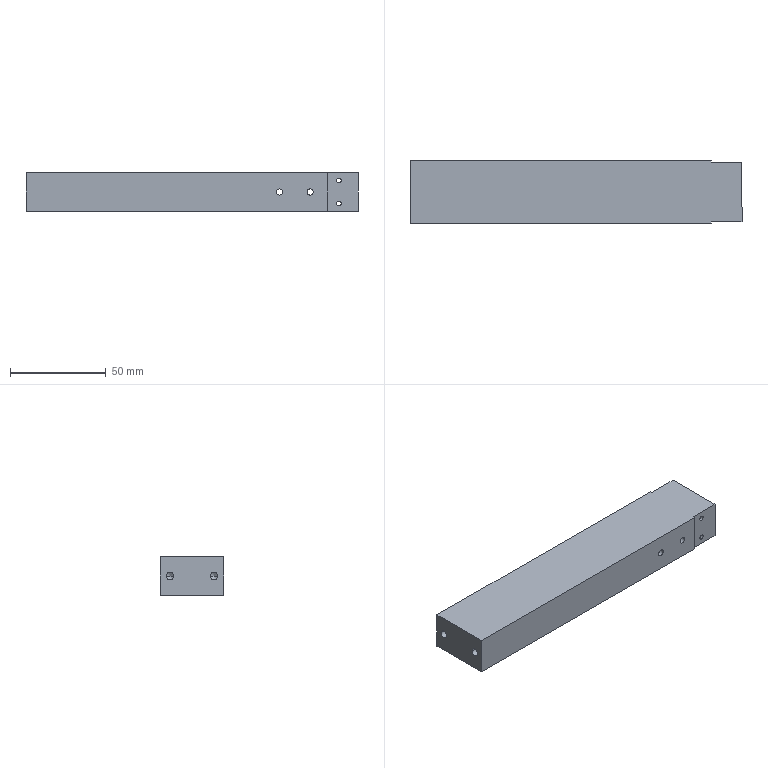Part | SolidWorks | features BaseBody 1 | 1 solid | 26 faces | box 173.5 x 33 x 20 mm | volume 112617 mm3 | cylinder 12 | plane 10 | cone 4 | commonest cylinder face diameters 2.459 x4 3.242 x4 4.134 x4
STEP:
#1=CARTESIAN_POINT('',(205.119,38.484,16.));
#2=VERTEX_POINT('',#1);
#3=CARTESIAN_POINT('',(207.578,38.484,16.));
#4=VERTEX_POINT('',#3);
#5=CARTESIAN_POINT('',(206.349,38.484,16.));
#6=DIRECTION('',(0.,-1.,0.));
#7=DIRECTION('',(-1.,0.,0.));
#8=AXIS2_PLACEMENT_3D('',#5,#6,#7);
#9=CIRCLE('',#8,1.229);
#10=EDGE_CURVE('',#2,#4,#9,.T.);
#11=ORIENTED_EDGE('',*,*,#10,.T.);
#12=CARTESIAN_POINT('',(207.578,69.484,16.));
#13=VERTEX_POINT('',#12);
#14=CARTESIAN_POINT('',(207.578,-107.255,16.));
#15=DIRECTION('',(0.,1.,0.));
#16=VECTOR('',#15,1000.);
#17=LINE('',#14,#16);
#18=EDGE_CURVE('',#4,#13,#17,.T.);
#19=ORIENTED_EDGE('',*,*,#18,.T.);
#20=CARTESIAN_POINT('',(205.119,69.484,16.));
#21=VERTEX_POINT('',#20);
#22=CARTESIAN_POINT('',(206.349,69.484,16.));
#23=DIRECTION('',(0.,-1.,0.));
#24=DIRECTION('',(-1.,0.,0.));
#25=AXIS2_PLACEMENT_3D('',#22,#23,#24);
#26=CIRCLE('',#25,1.229);
#27=EDGE_CURVE('',#21,#13,#26,.T.);
#28=ORIENTED_EDGE('',*,*,#27,.F.);
#29=CARTESIAN_POINT('',(205.119,-107.255,16.));
#30=DIRECTION('',(0.,1.,0.));
#31=VECTOR('',#30,1000.);
#32=LINE('',#29,#31);
#33=EDGE_CURVE('',#2,#21,#32,.T.);
#34=ORIENTED_EDGE('',*,*,#33,.F.);
#35=EDGE_LOOP('',(#11,#19,#28,#34));
#36=FACE_OUTER_BOUND('',#35,.T.);
#37=CARTESIAN_POINT('',(206.349,-107.255,16.));
#38=DIRECTION('',(0.,1.,0.));
#39=DIRECTION('',(-1.,0.,0.));
#40=AXIS2_PLACEMENT_3D('',#37,#38,#39);
#41=CYLINDRICAL_SURFACE('',#40,1.229);
#42=ADVANCED_FACE('',(#36),#41,.F.);
#43=CARTESIAN_POINT('',(205.119,38.484,4.));
#44=VERTEX_POINT('',#43);
#45=CARTESIAN_POINT('',(207.578,38.484,4.));
#46=VERTEX_POINT('',#45);
#47=CARTESIAN_POINT('',(206.349,38.484,4.));
#48=DIRECTION('',(0.,-1.,0.));
#49=DIRECTION('',(-1.,0.,0.));
#50=AXIS2_PLACEMENT_3D('',#47,#48,#49);
#51=CIRCLE('',#50,1.229);
#52=EDGE_CURVE('',#44,#46,#51,.T.);
#53=ORIENTED_EDGE('',*,*,#52,.T.);
#54=CARTESIAN_POINT('',(207.578,69.484,4.));
#55=VERTEX_POINT('',#54);
#56=CARTESIAN_POINT('',(207.578,-107.255,4.));
#57=DIRECTION('',(0.,1.,0.));
#58=VECTOR('',#57,1000.);
#59=LINE('',#56,#58);
#60=EDGE_CURVE('',#46,#55,#59,.T.);
#61=ORIENTED_EDGE('',*,*,#60,.T.);
#62=CARTESIAN_POINT('',(205.119,69.484,4.));
#63=VERTEX_POINT('',#62);
#64=CARTESIAN_POINT('',(206.349,69.484,4.));
#65=DIRECTION('',(0.,-1.,0.));
#66=DIRECTION('',(-1.,0.,0.));
#67=AXIS2_PLACEMENT_3D('',#64,#65,#66);
#68=CIRCLE('',#67,1.229);
#69=EDGE_CURVE('',#63,#55,#68,.T.);
#70=ORIENTED_EDGE('',*,*,#69,.F.);
#71=CARTESIAN_POINT('',(205.119,-107.255,4.));
#72=DIRECTION('',(0.,1.,0.));
#73=VECTOR('',#72,1000.);
#74=LINE('',#71,#73);
#75=EDGE_CURVE('',#44,#63,#74,.T.);
#76=ORIENTED_EDGE('',*,*,#75,.F.);
#77=EDGE_LOOP('',(#53,#61,#70,#76));
#78=FACE_OUTER_BOUND('',#77,.T.);
#79=CARTESIAN_POINT('',(206.349,-107.255,4.));
#80=DIRECTION('',(0.,1.,0.));
#81=DIRECTION('',(-1.,0.,0.));
#82=AXIS2_PLACEMENT_3D('',#79,#80,#81);
#83=CYLINDRICAL_SURFACE('',#82,1.229);
#84=ADVANCED_FACE('',(#78),#83,.F.);
#85=CARTESIAN_POINT('',(176.97,37.484,10.));
#86=VERTEX_POINT('',#85);
#87=CARTESIAN_POINT('',(173.728,37.484,10.));
#88=VERTEX_POINT('',#87);
#89=CARTESIAN_POINT('',(175.349,37.484,10.));
#90=DIRECTION('',(0.,1.,0.));
#91=DIRECTION('',(-1.,0.,0.));
#92=AXIS2_PLACEMENT_3D('',#89,#90,#91);
#93=CIRCLE('',#92,1.621);
#94=EDGE_CURVE('',#86,#88,#93,.T.);
#95=ORIENTED_EDGE('',*,*,#94,.F.);
#96=CARTESIAN_POINT('',(176.97,70.484,10.));
#97=VERTEX_POINT('',#96);
#98=CARTESIAN_POINT('',(176.97,-107.255,10.));
#99=DIRECTION('',(0.,1.,0.));
#100=VECTOR('',#99,1000.);
#101=LINE('',#98,#100);
#102=EDGE_CURVE('',#86,#97,#101,.T.);
#103=ORIENTED_EDGE('',*,*,#102,.T.);
#104=CARTESIAN_POINT('',(173.728,70.484,10.));
#105=VERTEX_POINT('',#104);
#106=CARTESIAN_POINT('',(175.349,70.484,10.));
#107=DIRECTION('',(0.,-1.,0.));
#108=DIRECTION('',(-1.,0.,0.));
#109=AXIS2_PLACEMENT_3D('',#106,#107,#108);
#110=CIRCLE('',#109,1.621);
#111=EDGE_CURVE('',#105,#97,#110,.T.);
#112=ORIENTED_EDGE('',*,*,#111,.F.);
#113=CARTESIAN_POINT('',(173.728,-107.255,10.));
#114=DIRECTION('',(0.,1.,0.));
#115=VECTOR('',#114,1000.);
#116=LINE('',#113,#115);
#117=EDGE_CURVE('',#88,#105,#116,.T.);
#118=ORIENTED_EDGE('',*,*,#117,.F.);
#119=EDGE_LOOP('',(#95,#103,#112,#118));
#120=FACE_OUTER_BOUND('',#119,.T.);
#121=CARTESIAN_POINT('',(175.349,-107.255,10.));
#122=DIRECTION('',(0.,1.,0.));
#123=DIRECTION('',(-1.,0.,0.));
#124=AXIS2_PLACEMENT_3D('',#121,#122,#123);
#125=CYLINDRICAL_SURFACE('',#124,1.621);
#126=ADVANCED_FACE('',(#120),#125,.F.);
#127=CARTESIAN_POINT('',(192.97,37.484,10.));
#128=VERTEX_POINT('',#127);
#129=CARTESIAN_POINT('',(189.728,37.484,10.));
#130=VERTEX_POINT('',#129);
#131=CARTESIAN_POINT('',(191.349,37.484,10.));
#132=DIRECTION('',(0.,1.,0.));
#133=DIRECTION('',(-1.,0.,0.));
#134=AXIS2_PLACEMENT_3D('',#131,#132,#133);
#135=CIRCLE('',#134,1.621);
#136=EDGE_CURVE('',#128,#130,#135,.T.);
#137=ORIENTED_EDGE('',*,*,#136,.F.);
#138=CARTESIAN_POINT('',(192.97,70.484,10.));
#139=VERTEX_POINT('',#138);
#140=CARTESIAN_POINT('',(192.97,-107.255,10.));
#141=DIRECTION('',(0.,1.,0.));
#142=VECTOR('',#141,1000.);
#143=LINE('',#140,#142);
#144=EDGE_CURVE('',#128,#139,#143,.T.);
#145=ORIENTED_EDGE('',*,*,#144,.T.);
#146=CARTESIAN_POINT('',(189.728,70.484,10.));
#147=VERTEX_POINT('',#146);
#148=CARTESIAN_POINT('',(191.349,70.484,10.));
#149=DIRECTION('',(0.,-1.,0.));
#150=DIRECTION('',(-1.,0.,0.));
#151=AXIS2_PLACEMENT_3D('',#148,#149,#150);
#152=CIRCLE('',#151,1.621);
#153=EDGE_CURVE('',#147,#139,#152,.T.);
#154=ORIENTED_EDGE('',*,*,#153,.F.);
#155=CARTESIAN_POINT('',(189.728,-107.255,10.));
#156=DIRECTION('',(0.,1.,0.));
#157=VECTOR('',#156,1000.);
#158=LINE('',#155,#157);
#159=EDGE_CURVE('',#130,#147,#158,.T.);
#160=ORIENTED_EDGE('',*,*,#159,.F.);
#161=EDGE_LOOP('',(#137,#145,#154,#160));
#162=FACE_OUTER_BOUND('',#161,.T.);
#163=CARTESIAN_POINT('',(191.349,-107.255,10.));
#164=DIRECTION('',(0.,1.,0.));
#165=DIRECTION('',(-1.,0.,0.));
#166=AXIS2_PLACEMENT_3D('',#163,#164,#165);
#167=CYLINDRICAL_SURFACE('',#166,1.621);
#168=ADVANCED_FACE('',(#162),#167,.F.);
#169=CARTESIAN_POINT('',(57.849,67.551,10.));
#170=VERTEX_POINT('',#169);
#171=CARTESIAN_POINT('',(57.849,63.417,10.));
#172=VERTEX_POINT('',#171);
#173=CARTESIAN_POINT('',(57.849,65.484,10.));
#174=DIRECTION('',(-1.,0.,0.));
#175=DIRECTION('',(0.,-1.,0.));
#176=AXIS2_PLACEMENT_3D('',#173,#174,#175);
#177=CIRCLE('',#176,2.067);
#178=EDGE_CURVE('',#170,#172,#177,.T.);
#179=ORIENTED_EDGE('',*,*,#178,.F.);
#180=CARTESIAN_POINT('',(42.849,67.551,10.));
#181=VERTEX_POINT('',#180);
#182=CARTESIAN_POINT('',(50.349,67.551,10.));
#183=DIRECTION('',(-1.,0.,0.));
#184=VECTOR('',#183,1000.);
#185=LINE('',#182,#184);
#186=EDGE_CURVE('',#170,#181,#185,.T.);
#187=ORIENTED_EDGE('',*,*,#186,.T.);
#188=CARTESIAN_POINT('',(42.849,63.417,10.));
#189=VERTEX_POINT('',#188);
#190=CARTESIAN_POINT('',(42.849,65.484,10.));
#191=DIRECTION('',(1.,0.,0.));
#192=DIRECTION('',(0.,-1.,0.));
#193=AXIS2_PLACEMENT_3D('',#190,#191,#192);
#194=CIRCLE('',#193,2.067);
#195=EDGE_CURVE('',#189,#181,#194,.T.);
#196=ORIENTED_EDGE('',*,*,#195,.F.);
#197=CARTESIAN_POINT('',(50.349,63.417,10.));
#198=DIRECTION('',(-1.,0.,0.));
#199=VECTOR('',#198,1000.);
#200=LINE('',#197,#199);
#201=EDGE_CURVE('',#172,#189,#200,.T.);
#202=ORIENTED_EDGE('',*,*,#201,.F.);
#203=EDGE_LOOP('',(#179,#187,#196,#202));
#204=FACE_OUTER_BOUND('',#203,.T.);
#205=CARTESIAN_POINT('',(50.349,65.484,10.));
#206=DIRECTION('',(-1.,0.,0.));
#207=DIRECTION('',(0.,-1.,0.));
#208=AXIS2_PLACEMENT_3D('',#205,#206,#207);
#209=CYLINDRICAL_SURFACE('',#208,2.067);
#210=ADVANCED_FACE('',(#204),#209,.F.);
#211=CARTESIAN_POINT('',(57.849,44.551,10.));
#212=VERTEX_POINT('',#211);
#213=CARTESIAN_POINT('',(57.849,40.417,10.));
#214=VERTEX_POINT('',#213);
#215=CARTESIAN_POINT('',(57.849,42.484,10.));
#216=DIRECTION('',(-1.,0.,0.));
#217=DIRECTION('',(0.,-1.,0.));
#218=AXIS2_PLACEMENT_3D('',#215,#216,#217);
#219=CIRCLE('',#218,2.067);
#220=EDGE_CURVE('',#212,#214,#219,.T.);
#221=ORIENTED_EDGE('',*,*,#220,.F.);
#222=CARTESIAN_POINT('',(42.849,44.551,10.));
#223=VERTEX_POINT('',#222);
#224=CARTESIAN_POINT('',(50.349,44.551,10.));
#225=DIRECTION('',(-1.,0.,0.));
#226=VECTOR('',#225,1000.);
#227=LINE('',#224,#226);
#228=EDGE_CURVE('',#212,#223,#227,.T.);
#229=ORIENTED_EDGE('',*,*,#228,.T.);
#230=CARTESIAN_POINT('',(42.849,40.417,10.));
#231=VERTEX_POINT('',#230);
#232=CARTESIAN_POINT('',(42.849,42.484,10.));
#233=DIRECTION('',(1.,0.,0.));
#234=DIRECTION('',(0.,-1.,0.));
#235=AXIS2_PLACEMENT_3D('',#232,#233,#234);
#236=CIRCLE('',#235,2.067);
#237=EDGE_CURVE('',#231,#223,#236,.T.);
#238=ORIENTED_EDGE('',*,*,#237,.F.);
#239=CARTESIAN_POINT('',(50.349,40.417,10.));
#240=DIRECTION('',(-1.,0.,0.));
#241=VECTOR('',#240,1000.);
#242=LINE('',#239,#241);
#243=EDGE_CURVE('',#214,#231,#242,.T.);
#244=ORIENTED_EDGE('',*,*,#243,.F.);
#245=EDGE_LOOP('',(#221,#229,#238,#244));
#246=FACE_OUTER_BOUND('',#245,.T.);
#247=CARTESIAN_POINT('',(50.349,42.484,10.));
#248=DIRECTION('',(-1.,0.,0.));
#249=DIRECTION('',(0.,-1.,0.));
#250=AXIS2_PLACEMENT_3D('',#247,#248,#249);
#251=CYLINDRICAL_SURFACE('',#250,2.067);
#252=ADVANCED_FACE('',(#246),#251,.F.);
#253=CARTESIAN_POINT('',(59.091,65.484,10.));
#254=VERTEX_POINT('',#253);
#255=CARTESIAN_POINT('',(57.849,63.417,10.));
#256=DIRECTION('',(-0.515,-0.8572,0.));
#257=VECTOR('',#256,1000.);
#258=LINE('',#255,#257);
#259=EDGE_CURVE('',#254,#172,#258,.T.);
#260=ORIENTED_EDGE('',*,*,#259,.F.);
#261=CARTESIAN_POINT('',(57.849,67.551,10.));
#262=DIRECTION('',(-0.515,0.8572,0.));
#263=VECTOR('',#262,1000.);
#264=LINE('',#261,#263);
#265=EDGE_CURVE('',#254,#170,#264,.T.);
#266=ORIENTED_EDGE('',*,*,#265,.T.);
#267=ORIENTED_EDGE('',*,*,#178,.T.);
#268=EDGE_LOOP('',(#260,#266,#267));
#269=FACE_OUTER_BOUND('',#268,.T.);
#270=CARTESIAN_POINT('',(57.849,65.484,10.));
#271=DIRECTION('',(-1.,0.,0.));
#272=DIRECTION('',(0.,-1.,0.));
#273=AXIS2_PLACEMENT_3D('',#270,#271,#272);
#274=CONICAL_SURFACE('',#273,2.067,1.03);
#275=ADVANCED_FACE('',(#269),#274,.F.);
#276=CARTESIAN_POINT('',(59.091,42.484,10.));
#277=VERTEX_POINT('',#276);
#278=CARTESIAN_POINT('',(57.849,40.417,10.));
#279=DIRECTION('',(-0.515,-0.8572,0.));
#280=VECTOR('',#279,1000.);
#281=LINE('',#278,#280);
#282=EDGE_CURVE('',#277,#214,#281,.T.);
#283=ORIENTED_EDGE('',*,*,#282,.F.);
#284=CARTESIAN_POINT('',(57.849,44.551,10.));
#285=DIRECTION('',(-0.515,0.8572,0.));
#286=VECTOR('',#285,1000.);
#287=LINE('',#284,#286);
#288=EDGE_CURVE('',#277,#212,#287,.T.);
#289=ORIENTED_EDGE('',*,*,#288,.T.);
#290=ORIENTED_EDGE('',*,*,#220,.T.);
#291=EDGE_LOOP('',(#283,#289,#290));
#292=FACE_OUTER_BOUND('',#291,.T.);
#293=CARTESIAN_POINT('',(57.849,42.484,10.));
#294=DIRECTION('',(-1.,0.,0.));
#295=DIRECTION('',(0.,-1.,0.));
#296=AXIS2_PLACEMENT_3D('',#293,#294,#295);
#297=CONICAL_SURFACE('',#296,2.067,1.03);
#298=ADVANCED_FACE('',(#292),#297,.F.);
#299=CARTESIAN_POINT('',(200.349,38.484,20.));
#300=VERTEX_POINT('',#299);
#301=CARTESIAN_POINT('',(216.349,38.484,20.));
#302=VERTEX_POINT('',#301);
#303=CARTESIAN_POINT('',(129.599,38.484,20.));
#304=DIRECTION('',(1.,0.,0.));
#305=VECTOR('',#304,1000.);
#306=LINE('',#303,#305);
#307=EDGE_CURVE('',#300,#302,#306,.T.);
#308=ORIENTED_EDGE('',*,*,#307,.T.);
#309=CARTESIAN_POINT('',(216.349,69.484,20.));
#310=VERTEX_POINT('',#309);
#311=CARTESIAN_POINT('',(216.349,53.984,20.));
#312=DIRECTION('',(0.,1.,0.));
#313=VECTOR('',#312,1000.);
#314=LINE('',#311,#313);
#315=EDGE_CURVE('',#302,#310,#314,.T.);
#316=ORIENTED_EDGE('',*,*,#315,.T.);
#317=CARTESIAN_POINT('',(200.349,69.484,20.));
#318=VERTEX_POINT('',#317);
#319=CARTESIAN_POINT('',(129.599,69.484,20.));
#320=DIRECTION('',(-1.,0.,0.));
#321=VECTOR('',#320,1000.);
#322=LINE('',#319,#321);
#323=EDGE_CURVE('',#310,#318,#322,.T.);
#324=ORIENTED_EDGE('',*,*,#323,.T.);
#325=CARTESIAN_POINT('',(200.349,70.484,20.));
#326=VERTEX_POINT('',#325);
#327=CARTESIAN_POINT('',(200.349,70.484,20.));
#328=DIRECTION('',(0.,1.,0.));
#329=VECTOR('',#328,1000.);
#330=LINE('',#327,#329);
#331=EDGE_CURVE('',#318,#326,#330,.T.);
#332=ORIENTED_EDGE('',*,*,#331,.T.);
#333=CARTESIAN_POINT('',(42.849,70.484,20.));
#334=VERTEX_POINT('',#333);
#335=CARTESIAN_POINT('',(129.599,70.484,20.));
#336=DIRECTION('',(-1.,0.,0.));
#337=VECTOR('',#336,1000.);
#338=LINE('',#335,#337);
#339=EDGE_CURVE('',#326,#334,#338,.T.);
#340=ORIENTED_EDGE('',*,*,#339,.T.);
#341=CARTESIAN_POINT('',(42.849,37.484,20.));
#342=VERTEX_POINT('',#341);
#343=CARTESIAN_POINT('',(42.849,53.984,20.));
#344=DIRECTION('',(0.,-1.,0.));
#345=VECTOR('',#344,1000.);
#346=LINE('',#343,#345);
#347=EDGE_CURVE('',#334,#342,#346,.T.);
#348=ORIENTED_EDGE('',*,*,#347,.T.);
#349=CARTESIAN_POINT('',(200.349,37.484,20.));
#350=VERTEX_POINT('',#349);
#351=CARTESIAN_POINT('',(129.599,37.484,20.));
#352=DIRECTION('',(1.,0.,0.));
#353=VECTOR('',#352,1000.);
#354=LINE('',#351,#353);
#355=EDGE_CURVE('',#342,#350,#354,.T.);
#356=ORIENTED_EDGE('',*,*,#355,.T.);
#357=CARTESIAN_POINT('',(200.349,37.484,20.));
#358=DIRECTION('',(0.,1.,0.));
#359=VECTOR('',#358,1000.);
#360=LINE('',#357,#359);
#361=EDGE_CURVE('',#350,#300,#360,.T.);
#362=ORIENTED_EDGE('',*,*,#361,.T.);
#363=EDGE_LOOP('',(#308,#316,#324,#332,#340,#348,#356,#362));
#364=FACE_OUTER_BOUND('',#363,.T.);
#365=CARTESIAN_POINT('',(129.599,53.984,20.));
#366=DIRECTION('',(0.,0.,1.));
#367=DIRECTION('',(1.,0.,0.));
#368=AXIS2_PLACEMENT_3D('',#365,#366,#367);
#369=PLANE('',#368);
#370=ADVANCED_FACE('',(#364),#369,.T.);
#371=CARTESIAN_POINT('',(216.349,38.484,0.));
#372=VERTEX_POINT('',#371);
#373=CARTESIAN_POINT('',(216.349,38.484,0.));
#374=DIRECTION('',(0.,0.,-1.));
#375=VECTOR('',#374,1000.);
#376=LINE('',#373,#375);
#377=EDGE_CURVE('',#302,#372,#376,.T.);
#378=ORIENTED_EDGE('',*,*,#377,.T.);
#379=CARTESIAN_POINT('',(216.349,69.484,0.));
#380=VERTEX_POINT('',#379);
#381=CARTESIAN_POINT('',(216.349,70.484,0.));
#382=DIRECTION('',(0.,1.,0.));
#383=VECTOR('',#382,1000.);
#384=LINE('',#381,#383);
#385=EDGE_CURVE('',#372,#380,#384,.T.);
#386=ORIENTED_EDGE('',*,*,#385,.T.);
#387=CARTESIAN_POINT('',(216.349,69.484,0.));
#388=DIRECTION('',(0.,0.,1.));
#389=VECTOR('',#388,1000.);
#390=LINE('',#387,#389);
#391=EDGE_CURVE('',#380,#310,#390,.T.);
#392=ORIENTED_EDGE('',*,*,#391,.T.);
#393=ORIENTED_EDGE('',*,*,#315,.F.);
#394=EDGE_LOOP('',(#378,#386,#392,#393));
#395=FACE_OUTER_BOUND('',#394,.T.);
#396=CARTESIAN_POINT('',(216.349,70.484,0.));
#397=DIRECTION('',(1.,0.,0.));
#398=DIRECTION('',(0.,0.,-1.));
#399=AXIS2_PLACEMENT_3D('',#396,#397,#398);
#400=PLANE('',#399);
#401=ADVANCED_FACE('',(#395),#400,.T.);
#402=ORIENTED_EDGE('',*,*,#10,.F.);
#403=CARTESIAN_POINT('',(206.349,38.484,16.));
#404=DIRECTION('',(0.,-1.,0.));
#405=DIRECTION('',(-1.,0.,0.));
#406=AXIS2_PLACEMENT_3D('',#403,#404,#405);
#407=CIRCLE('',#406,1.229);
#408=EDGE_CURVE('',#4,#2,#407,.T.);
#409=ORIENTED_EDGE('',*,*,#408,.F.);
#410=EDGE_LOOP('',(#402,#409));
#411=FACE_BOUND('',#410,.T.);
#412=ORIENTED_EDGE('',*,*,#52,.F.);
#413=CARTESIAN_POINT('',(206.349,38.484,4.));
#414=DIRECTION('',(0.,-1.,0.));
#415=DIRECTION('',(-1.,0.,0.));
#416=AXIS2_PLACEMENT_3D('',#413,#414,#415);
#417=CIRCLE('',#416,1.229);
#418=EDGE_CURVE('',#46,#44,#417,.T.);
#419=ORIENTED_EDGE('',*,*,#418,.F.);
#420=EDGE_LOOP('',(#412,#419));
#421=FACE_BOUND('',#420,.T.);
#422=CARTESIAN_POINT('',(200.349,38.484,0.));
#423=VERTEX_POINT('',#422);
#424=CARTESIAN_POINT('',(208.349,38.484,0.));
#425=DIRECTION('',(-1.,0.,0.));
#426=VECTOR('',#425,1000.);
#427=LINE('',#424,#426);
#428=EDGE_CURVE('',#372,#423,#427,.T.);
#429=ORIENTED_EDGE('',*,*,#428,.F.);
#430=ORIENTED_EDGE('',*,*,#377,.F.);
#431=ORIENTED_EDGE('',*,*,#307,.F.);
#432=CARTESIAN_POINT('',(200.349,38.484,10.));
#433=DIRECTION('',(0.,0.,1.));
#434=VECTOR('',#433,1000.);
#435=LINE('',#432,#434);
#436=EDGE_CURVE('',#423,#300,#435,.T.);
#437=ORIENTED_EDGE('',*,*,#436,.F.);
#438=EDGE_LOOP('',(#429,#430,#431,#437));
#439=FACE_OUTER_BOUND('',#438,.T.);
#440=CARTESIAN_POINT('',(208.349,38.484,10.));
#441=DIRECTION('',(0.,1.,0.));
#442=DIRECTION('',(0.,0.,1.));
#443=AXIS2_PLACEMENT_3D('',#440,#441,#442);
#444=PLANE('',#443);
#445=ADVANCED_FACE('',(#411,#421,#439),#444,.F.);
#446=CARTESIAN_POINT('',(175.349,37.484,10.));
#447=DIRECTION('',(0.,1.,0.));
#448=DIRECTION('',(-1.,0.,0.));
#449=AXIS2_PLACEMENT_3D('',#446,#447,#448);
#450=CIRCLE('',#449,1.621);
#451=EDGE_CURVE('',#88,#86,#450,.T.);
#452=ORIENTED_EDGE('',*,*,#451,.T.);
#453=ORIENTED_EDGE('',*,*,#94,.T.);
#454=EDGE_LOOP('',(#452,#453));
#455=FACE_BOUND('',#454,.T.);
#456=CARTESIAN_POINT('',(191.349,37.484,10.));
#457=DIRECTION('',(0.,1.,0.));
#458=DIRECTION('',(-1.,0.,0.));
#459=AXIS2_PLACEMENT_3D('',#456,#457,#458);
#460=CIRCLE('',#459,1.621);
#461=EDGE_CURVE('',#130,#128,#460,.T.);
#462=ORIENTED_EDGE('',*,*,#461,.T.);
#463=ORIENTED_EDGE('',*,*,#136,.T.);
#464=EDGE_LOOP('',(#462,#463));
#465=FACE_BOUND('',#464,.T.);
#466=CARTESIAN_POINT('',(42.849,37.484,0.));
#467=VERTEX_POINT('',#466);
#468=CARTESIAN_POINT('',(42.849,37.484,0.));
#469=DIRECTION('',(0.,0.,-1.));
#470=VECTOR('',#469,1000.);
#471=LINE('',#468,#470);
#472=EDGE_CURVE('',#342,#467,#471,.T.);
#473=ORIENTED_EDGE('',*,*,#472,.T.);
#474=CARTESIAN_POINT('',(200.349,37.484,0.));
#475=VERTEX_POINT('',#474);
#476=CARTESIAN_POINT('',(216.349,37.484,0.));
#477=DIRECTION('',(1.,0.,0.));
#478=VECTOR('',#477,1000.);
#479=LINE('',#476,#478);
#480=EDGE_CURVE('',#467,#475,#479,.T.);
#481=ORIENTED_EDGE('',*,*,#480,.T.);
#482=CARTESIAN_POINT('',(200.349,37.484,0.));
#483=DIRECTION('',(0.,0.,1.));
#484=VECTOR('',#483,1000.);
#485=LINE('',#482,#484);
#486=EDGE_CURVE('',#475,#350,#485,.T.);
#487=ORIENTED_EDGE('',*,*,#486,.T.);
#488=ORIENTED_EDGE('',*,*,#355,.F.);
#489=EDGE_LOOP('',(#473,#481,#487,#488));
#490=FACE_OUTER_BOUND('',#489,.T.);
#491=CARTESIAN_POINT('',(216.349,37.484,0.));
#492=DIRECTION('',(0.,-1.,0.));
#493=DIRECTION('',(0.,0.,-1.));
#494=AXIS2_PLACEMENT_3D('',#491,#492,#493);
#495=PLANE('',#494);
#496=ADVANCED_FACE('',(#455,#465,#490),#495,.T.);
#497=ORIENTED_EDGE('',*,*,#195,.T.);
#498=CARTESIAN_POINT('',(42.849,65.484,10.));
#499=DIRECTION('',(1.,0.,0.));
#500=DIRECTION('',(0.,-1.,0.));
#501=AXIS2_PLACEMENT_3D('',#498,#499,#500);
#502=CIRCLE('',#501,2.067);
#503=EDGE_CURVE('',#181,#189,#502,.T.);
#504=ORIENTED_EDGE('',*,*,#503,.T.);
#505=EDGE_LOOP('',(#497,#504));
#506=FACE_BOUND('',#505,.T.);
#507=ORIENTED_EDGE('',*,*,#237,.T.);
#508=CARTESIAN_POINT('',(42.849,42.484,10.));
#509=DIRECTION('',(1.,0.,0.));
#510=DIRECTION('',(0.,-1.,0.));
#511=AXIS2_PLACEMENT_3D('',#508,#509,#510);
#512=CIRCLE('',#511,2.067);
#513=EDGE_CURVE('',#223,#231,#512,.T.);
#514=ORIENTED_EDGE('',*,*,#513,.T.);
#515=EDGE_LOOP('',(#507,#514));
#516=FACE_BOUND('',#515,.T.);
#517=CARTESIAN_POINT('',(42.849,70.484,0.));
#518=VERTEX_POINT('',#517);
#519=CARTESIAN_POINT('',(42.849,37.484,0.));
#520=DIRECTION('',(0.,-1.,0.));
#521=VECTOR('',#520,1000.);
#522=LINE('',#519,#521);
#523=EDGE_CURVE('',#518,#467,#522,.T.);
#524=ORIENTED_EDGE('',*,*,#523,.T.);
#525=ORIENTED_EDGE('',*,*,#472,.F.);
#526=ORIENTED_EDGE('',*,*,#347,.F.);
#527=CARTESIAN_POINT('',(42.849,70.484,0.));
#528=DIRECTION('',(0.,0.,-1.));
#529=VECTOR('',#528,1000.);
#530=LINE('',#527,#529);
#531=EDGE_CURVE('',#334,#518,#530,.T.);
#532=ORIENTED_EDGE('',*,*,#531,.T.);
#533=EDGE_LOOP('',(#524,#525,#526,#532));
#534=FACE_OUTER_BOUND('',#533,.T.);
#535=CARTESIAN_POINT('',(42.849,37.484,0.));
#536=DIRECTION('',(-1.,0.,0.));
#537=DIRECTION('',(0.,0.,1.));
#538=AXIS2_PLACEMENT_3D('',#535,#536,#537);
#539=PLANE('',#538);
#540=ADVANCED_FACE('',(#506,#516,#534),#539,.T.);
#541=ORIENTED_EDGE('',*,*,#111,.T.);
#542=CARTESIAN_POINT('',(175.349,70.484,10.));
#543=DIRECTION('',(0.,-1.,0.));
#544=DIRECTION('',(-1.,0.,0.));
#545=AXIS2_PLACEMENT_3D('',#542,#543,#544);
#546=CIRCLE('',#545,1.621);
#547=EDGE_CURVE('',#97,#105,#546,.T.);
#548=ORIENTED_EDGE('',*,*,#547,.T.);
#549=EDGE_LOOP('',(#541,#548));
#550=FACE_BOUND('',#549,.T.);
#551=ORIENTED_EDGE('',*,*,#153,.T.);
#552=CARTESIAN_POINT('',(191.349,70.484,10.));
#553=DIRECTION('',(0.,-1.,0.));
#554=DIRECTION('',(-1.,0.,0.));
#555=AXIS2_PLACEMENT_3D('',#552,#553,#554);
#556=CIRCLE('',#555,1.621);
#557=EDGE_CURVE('',#139,#147,#556,.T.);
#558=ORIENTED_EDGE('',*,*,#557,.T.);
#559=EDGE_LOOP('',(#551,#558));
#560=FACE_BOUND('',#559,.T.);
#561=ORIENTED_EDGE('',*,*,#531,.F.);
#562=ORIENTED_EDGE('',*,*,#339,.F.);
#563=CARTESIAN_POINT('',(200.349,70.484,0.));
#564=VERTEX_POINT('',#563);
#565=CARTESIAN_POINT('',(200.349,70.484,0.));
#566=DIRECTION('',(0.,0.,-1.));
#567=VECTOR('',#566,1000.);
#568=LINE('',#565,#567);
#569=EDGE_CURVE('',#326,#564,#568,.T.);
#570=ORIENTED_EDGE('',*,*,#569,.T.);
#571=CARTESIAN_POINT('',(42.849,70.484,0.));
#572=DIRECTION('',(-1.,0.,0.));
#573=VECTOR('',#572,1000.);
#574=LINE('',#571,#573);
#575=EDGE_CURVE('',#564,#518,#574,.T.);
#576=ORIENTED_EDGE('',*,*,#575,.T.);
#577=EDGE_LOOP('',(#561,#562,#570,#576));
#578=FACE_OUTER_BOUND('',#577,.T.);
#579=CARTESIAN_POINT('',(42.849,70.484,0.));
#580=DIRECTION('',(0.,1.,0.));
#581=DIRECTION('',(0.,0.,1.));
#582=AXIS2_PLACEMENT_3D('',#579,#580,#581);
#583=PLANE('',#582);
#584=ADVANCED_FACE('',(#550,#560,#578),#583,.T.);
#585=ORIENTED_EDGE('',*,*,#27,.T.);
#586=CARTESIAN_POINT('',(206.349,69.484,16.));
#587=DIRECTION('',(0.,-1.,0.));
#588=DIRECTION('',(-1.,0.,0.));
#589=AXIS2_PLACEMENT_3D('',#586,#587,#588);
#590=CIRCLE('',#589,1.229);
#591=EDGE_CURVE('',#13,#21,#590,.T.);
#592=ORIENTED_EDGE('',*,*,#591,.T.);
#593=EDGE_LOOP('',(#585,#592));
#594=FACE_BOUND('',#593,.T.);
#595=ORIENTED_EDGE('',*,*,#69,.T.);
#596=CARTESIAN_POINT('',(206.349,69.484,4.));
#597=DIRECTION('',(0.,-1.,0.));
#598=DIRECTION('',(-1.,0.,0.));
#599=AXIS2_PLACEMENT_3D('',#596,#597,#598);
#600=CIRCLE('',#599,1.229);
#601=EDGE_CURVE('',#55,#63,#600,.T.);
#602=ORIENTED_EDGE('',*,*,#601,.T.);
#603=EDGE_LOOP('',(#595,#602));
#604=FACE_BOUND('',#603,.T.);
#605=CARTESIAN_POINT('',(200.349,69.484,0.));
#606=VERTEX_POINT('',#605);
#607=CARTESIAN_POINT('',(200.349,69.484,10.));
#608=DIRECTION('',(0.,0.,1.));
#609=VECTOR('',#608,1000.);
#610=LINE('',#607,#609);
#611=EDGE_CURVE('',#606,#318,#610,.T.);
#612=ORIENTED_EDGE('',*,*,#611,.T.);
#613=ORIENTED_EDGE('',*,*,#323,.F.);
#614=ORIENTED_EDGE('',*,*,#391,.F.);
#615=CARTESIAN_POINT('',(208.349,69.484,0.));
#616=DIRECTION('',(-1.,0.,0.));
#617=VECTOR('',#616,1000.);
#618=LINE('',#615,#617);
#619=EDGE_CURVE('',#380,#606,#618,.T.);
#620=ORIENTED_EDGE('',*,*,#619,.T.);
#621=EDGE_LOOP('',(#612,#613,#614,#620));
#622=FACE_OUTER_BOUND('',#621,.T.);
#623=CARTESIAN_POINT('',(208.349,69.484,10.));
#624=DIRECTION('',(0.,1.,0.));
#625=DIRECTION('',(0.,0.,1.));
#626=AXIS2_PLACEMENT_3D('',#623,#624,#625);
#627=PLANE('',#626);
#628=ADVANCED_FACE('',(#594,#604,#622),#627,.T.);
#629=ORIENTED_EDGE('',*,*,#385,.F.);
#630=ORIENTED_EDGE('',*,*,#428,.T.);
#631=CARTESIAN_POINT('',(200.349,53.984,0.));
#632=DIRECTION('',(0.,1.,0.));
#633=VECTOR('',#632,1000.);
#634=LINE('',#631,#633);
#635=EDGE_CURVE('',#475,#423,#634,.T.);
#636=ORIENTED_EDGE('',*,*,#635,.F.);
#637=ORIENTED_EDGE('',*,*,#480,.F.);
#638=ORIENTED_EDGE('',*,*,#523,.F.);
#639=ORIENTED_EDGE('',*,*,#575,.F.);
#640=CARTESIAN_POINT('',(200.349,53.984,0.));
#641=DIRECTION('',(0.,1.,0.));
#642=VECTOR('',#641,1000.);
#643=LINE('',#640,#642);
#644=EDGE_CURVE('',#606,#564,#643,.T.);
#645=ORIENTED_EDGE('',*,*,#644,.F.);
#646=ORIENTED_EDGE('',*,*,#619,.F.);
#647=EDGE_LOOP('',(#629,#630,#636,#637,#638,#639,#645,#646));
#648=FACE_OUTER_BOUND('',#647,.T.);
#649=CARTESIAN_POINT('',(129.599,53.984,0.));
#650=DIRECTION('',(0.,0.,1.));
#651=DIRECTION('',(1.,0.,0.));
#652=AXIS2_PLACEMENT_3D('',#649,#650,#651);
#653=PLANE('',#652);
#654=ADVANCED_FACE('',(#648),#653,.F.);
#655=ORIENTED_EDGE('',*,*,#18,.F.);
#656=ORIENTED_EDGE('',*,*,#408,.T.);
#657=ORIENTED_EDGE('',*,*,#33,.T.);
#658=ORIENTED_EDGE('',*,*,#591,.F.);
#659=EDGE_LOOP('',(#655,#656,#657,#658));
#660=FACE_OUTER_BOUND('',#659,.T.);
#661=CARTESIAN_POINT('',(206.349,-107.255,16.));
#662=DIRECTION('',(0.,1.,0.));
#663=DIRECTION('',(-1.,0.,0.));
#664=AXIS2_PLACEMENT_3D('',#661,#662,#663);
#665=CYLINDRICAL_SURFACE('',#664,1.229);
#666=ADVANCED_FACE('',(#660),#665,.F.);
#667=ORIENTED_EDGE('',*,*,#60,.F.);
#668=ORIENTED_EDGE('',*,*,#418,.T.);
#669=ORIENTED_EDGE('',*,*,#75,.T.);
#670=ORIENTED_EDGE('',*,*,#601,.F.);
#671=EDGE_LOOP('',(#667,#668,#669,#670));
#672=FACE_OUTER_BOUND('',#671,.T.);
#673=CARTESIAN_POINT('',(206.349,-107.255,4.));
#674=DIRECTION('',(0.,1.,0.));
#675=DIRECTION('',(-1.,0.,0.));
#676=AXIS2_PLACEMENT_3D('',#673,#674,#675);
#677=CYLINDRICAL_SURFACE('',#676,1.229);
#678=ADVANCED_FACE('',(#672),#677,.F.);
#679=ORIENTED_EDGE('',*,*,#361,.F.);
#680=ORIENTED_EDGE('',*,*,#486,.F.);
#681=ORIENTED_EDGE('',*,*,#635,.T.);
#682=ORIENTED_EDGE('',*,*,#436,.T.);
#683=EDGE_LOOP('',(#679,#680,#681,#682));
#684=FACE_OUTER_BOUND('',#683,.T.);
#685=CARTESIAN_POINT('',(200.349,37.484,20.));
#686=DIRECTION('',(-1.,0.,0.));
#687=DIRECTION('',(0.,0.,1.));
#688=AXIS2_PLACEMENT_3D('',#685,#686,#687);
#689=PLANE('',#688);
#690=ADVANCED_FACE('',(#684),#689,.F.);
#691=ORIENTED_EDGE('',*,*,#102,.F.);
#692=ORIENTED_EDGE('',*,*,#451,.F.);
#693=ORIENTED_EDGE('',*,*,#117,.T.);
#694=ORIENTED_EDGE('',*,*,#547,.F.);
#695=EDGE_LOOP('',(#691,#692,#693,#694));
#696=FACE_OUTER_BOUND('',#695,.T.);
#697=CARTESIAN_POINT('',(175.349,-107.255,10.));
#698=DIRECTION('',(0.,1.,0.));
#699=DIRECTION('',(-1.,0.,0.));
#700=AXIS2_PLACEMENT_3D('',#697,#698,#699);
#701=CYLINDRICAL_SURFACE('',#700,1.621);
#702=ADVANCED_FACE('',(#696),#701,.F.);
#703=ORIENTED_EDGE('',*,*,#144,.F.);
#704=ORIENTED_EDGE('',*,*,#461,.F.);
#705=ORIENTED_EDGE('',*,*,#159,.T.);
#706=ORIENTED_EDGE('',*,*,#557,.F.);
#707=EDGE_LOOP('',(#703,#704,#705,#706));
#708=FACE_OUTER_BOUND('',#707,.T.);
#709=CARTESIAN_POINT('',(191.349,-107.255,10.));
#710=DIRECTION('',(0.,1.,0.));
#711=DIRECTION('',(-1.,0.,0.));
#712=AXIS2_PLACEMENT_3D('',#709,#710,#711);
#713=CYLINDRICAL_SURFACE('',#712,1.621);
#714=ADVANCED_FACE('',(#708),#713,.F.);
#715=ORIENTED_EDGE('',*,*,#186,.F.);
#716=CARTESIAN_POINT('',(57.849,65.484,10.));
#717=DIRECTION('',(-1.,0.,0.));
#718=DIRECTION('',(0.,-1.,0.));
#719=AXIS2_PLACEMENT_3D('',#716,#717,#718);
#720=CIRCLE('',#719,2.067);
#721=EDGE_CURVE('',#172,#170,#720,.T.);
#722=ORIENTED_EDGE('',*,*,#721,.F.);
#723=ORIENTED_EDGE('',*,*,#201,.T.);
#724=ORIENTED_EDGE('',*,*,#503,.F.);
#725=EDGE_LOOP('',(#715,#722,#723,#724));
#726=FACE_OUTER_BOUND('',#725,.T.);
#727=CARTESIAN_POINT('',(50.349,65.484,10.));
#728=DIRECTION('',(-1.,0.,0.));
#729=DIRECTION('',(0.,-1.,0.));
#730=AXIS2_PLACEMENT_3D('',#727,#728,#729);
#731=CYLINDRICAL_SURFACE('',#730,2.067);
#732=ADVANCED_FACE('',(#726),#731,.F.);
#733=ORIENTED_EDGE('',*,*,#228,.F.);
#734=CARTESIAN_POINT('',(57.849,42.484,10.));
#735=DIRECTION('',(-1.,0.,0.));
#736=DIRECTION('',(0.,-1.,0.));
#737=AXIS2_PLACEMENT_3D('',#734,#735,#736);
#738=CIRCLE('',#737,2.067);
#739=EDGE_CURVE('',#214,#212,#738,.T.);
#740=ORIENTED_EDGE('',*,*,#739,.F.);
#741=ORIENTED_EDGE('',*,*,#243,.T.);
#742=ORIENTED_EDGE('',*,*,#513,.F.);
#743=EDGE_LOOP('',(#733,#740,#741,#742));
#744=FACE_OUTER_BOUND('',#743,.T.);
#745=CARTESIAN_POINT('',(50.349,42.484,10.));
#746=DIRECTION('',(-1.,0.,0.));
#747=DIRECTION('',(0.,-1.,0.));
#748=AXIS2_PLACEMENT_3D('',#745,#746,#747);
#749=CYLINDRICAL_SURFACE('',#748,2.067);
#750=ADVANCED_FACE('',(#744),#749,.F.);
#751=ORIENTED_EDGE('',*,*,#644,.T.);
#752=ORIENTED_EDGE('',*,*,#569,.F.);
#753=ORIENTED_EDGE('',*,*,#331,.F.);
#754=ORIENTED_EDGE('',*,*,#611,.F.);
#755=EDGE_LOOP('',(#751,#752,#753,#754));
#756=FACE_OUTER_BOUND('',#755,.T.);
#757=CARTESIAN_POINT('',(200.349,70.484,0.));
#758=DIRECTION('',(-1.,0.,0.));
#759=DIRECTION('',(0.,0.,1.));
#760=AXIS2_PLACEMENT_3D('',#757,#758,#759);
#761=PLANE('',#760);
#762=ADVANCED_FACE('',(#756),#761,.F.);
#763=ORIENTED_EDGE('',*,*,#265,.F.);
#764=ORIENTED_EDGE('',*,*,#259,.T.);
#765=ORIENTED_EDGE('',*,*,#721,.T.);
#766=EDGE_LOOP('',(#763,#764,#765));
#767=FACE_OUTER_BOUND('',#766,.T.);
#768=CARTESIAN_POINT('',(57.849,65.484,10.));
#769=DIRECTION('',(-1.,0.,0.));
#770=DIRECTION('',(0.,-1.,0.));
#771=AXIS2_PLACEMENT_3D('',#768,#769,#770);
#772=CONICAL_SURFACE('',#771,2.067,1.03);
#773=ADVANCED_FACE('',(#767),#772,.F.);
#774=ORIENTED_EDGE('',*,*,#288,.F.);
#775=ORIENTED_EDGE('',*,*,#282,.T.);
#776=ORIENTED_EDGE('',*,*,#739,.T.);
#777=EDGE_LOOP('',(#774,#775,#776));
#778=FACE_OUTER_BOUND('',#777,.T.);
#779=CARTESIAN_POINT('',(57.849,42.484,10.));
#780=DIRECTION('',(-1.,0.,0.));
#781=DIRECTION('',(0.,-1.,0.));
#782=AXIS2_PLACEMENT_3D('',#779,#780,#781);
#783=CONICAL_SURFACE('',#782,2.067,1.03);
#784=ADVANCED_FACE('',(#778),#783,.F.);
#785=CLOSED_SHELL('',(#42,#84,#126,#168,#210,#252,#275,#298,#370,#401,#445,#496,#540,#584,#628,#654,#666,#678,#690,#702,#714,#732,#750,#762,#773,#784));
#786=MANIFOLD_SOLID_BREP('',#785);
#787=CARTESIAN_POINT('',(0.,0.,0.));
#788=DIRECTION('',(0.,0.,1.));
#789=DIRECTION('',(1.,0.,0.));
#790=AXIS2_PLACEMENT_3D('',#787,#788,#789);
#791=(LENGTH_UNIT()NAMED_UNIT(*)SI_UNIT(.MILLI.,.METRE.));
#792=UNCERTAINTY_MEASURE_WITH_UNIT(LENGTH_MEASURE(0.00001),#791,'','');
#793=(NAMED_UNIT(*)PLANE_ANGLE_UNIT()SI_UNIT($,.RADIAN.));
#794=(NAMED_UNIT(*)SI_UNIT($,.STERADIAN.)SOLID_ANGLE_UNIT());
#795=(GEOMETRIC_REPRESENTATION_CONTEXT(3)GLOBAL_UNCERTAINTY_ASSIGNED_CONTEXT((#792))GLOBAL_UNIT_ASSIGNED_CONTEXT((#791,#793,#794))REPRESENTATION_CONTEXT('',''));
#796=ADVANCED_BREP_SHAPE_REPRESENTATION('',(#786,#790),#795);